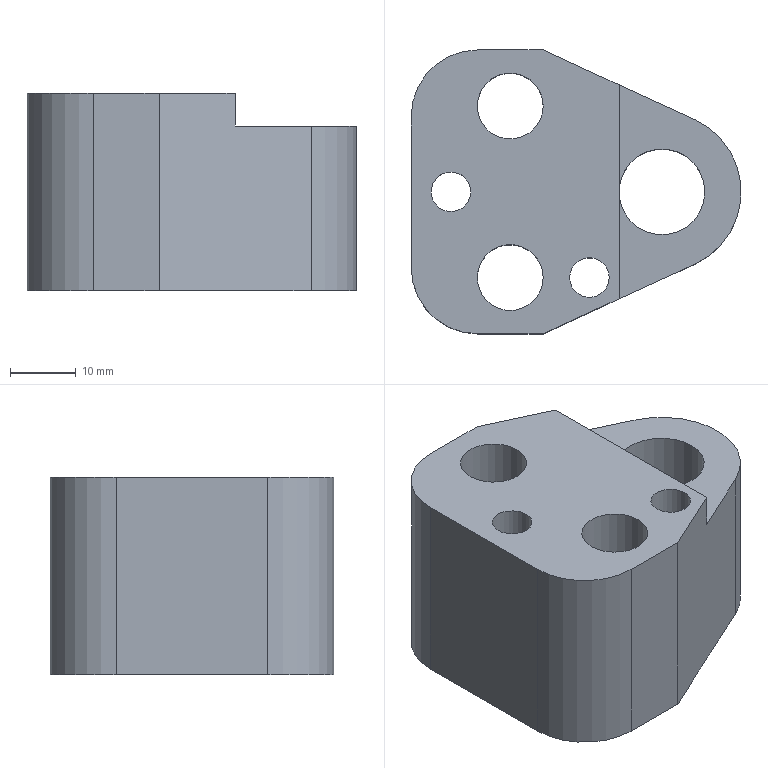Part | NX | features solid 2 | 1 solid | 25 faces | box 50 x 43 x 30 mm | volume 35945 mm3 | plane 13 | cylinder 12 | commonest cylinder face diameters 6 x2 8 x2 10 x2 14 x2 20 x2 13 x1
STEP:
#1=CARTESIAN_POINT('',(-1290.413,384.928,103.));
#2=VERTEX_POINT('',#1);
#3=CARTESIAN_POINT('',(-1294.413,384.928,103.));
#4=DIRECTION('',(0.,0.,1.));
#5=DIRECTION('',(1.,0.,0.));
#6=AXIS2_PLACEMENT_3D('',#3,#4,#5);
#7=CIRCLE('',#6,4.);
#8=EDGE_CURVE('',#2,#2,#7,.F.);
#9=ORIENTED_EDGE('',*,*,#8,.F.);
#10=EDGE_LOOP('',(#9));
#11=FACE_BOUND('',#10,.T.);
#12=CARTESIAN_POINT('',(-1292.413,371.928,103.));
#13=VERTEX_POINT('',#12);
#14=CARTESIAN_POINT('',(-1285.413,371.928,103.));
#15=DIRECTION('',(0.,0.,-1.));
#16=DIRECTION('',(-1.,0.,0.));
#17=AXIS2_PLACEMENT_3D('',#14,#15,#16);
#18=CIRCLE('',#17,7.);
#19=EDGE_CURVE('',#13,#13,#18,.T.);
#20=ORIENTED_EDGE('',*,*,#19,.F.);
#21=EDGE_LOOP('',(#20));
#22=FACE_BOUND('',#21,.T.);
#23=CARTESIAN_POINT('',(-1292.413,397.928,103.));
#24=VERTEX_POINT('',#23);
#25=CARTESIAN_POINT('',(-1285.413,397.928,103.));
#26=DIRECTION('',(0.,0.,-1.));
#27=DIRECTION('',(-1.,0.,0.));
#28=AXIS2_PLACEMENT_3D('',#25,#26,#27);
#29=CIRCLE('',#28,7.);
#30=EDGE_CURVE('',#24,#24,#29,.T.);
#31=ORIENTED_EDGE('',*,*,#30,.F.);
#32=EDGE_LOOP('',(#31));
#33=FACE_BOUND('',#32,.T.);
#34=CARTESIAN_POINT('',(-1255.913,384.928,103.));
#35=VERTEX_POINT('',#34);
#36=CARTESIAN_POINT('',(-1262.413,384.928,103.));
#37=DIRECTION('',(0.,0.,1.));
#38=DIRECTION('',(1.,0.,0.));
#39=AXIS2_PLACEMENT_3D('',#36,#37,#38);
#40=CIRCLE('',#39,6.5);
#41=EDGE_CURVE('',#35,#35,#40,.T.);
#42=ORIENTED_EDGE('',*,*,#41,.T.);
#43=EDGE_LOOP('',(#42));
#44=FACE_BOUND('',#43,.T.);
#45=CARTESIAN_POINT('',(-1257.394,395.828,103.));
#46=VERTEX_POINT('',#45);
#47=CARTESIAN_POINT('',(-1280.413,406.428,103.));
#48=VERTEX_POINT('',#47);
#49=CARTESIAN_POINT('',(-1257.394,395.828,103.));
#50=DIRECTION('',(-0.9083,0.4183,0.));
#51=VECTOR('',#50,1000.);
#52=LINE('',#49,#51);
#53=EDGE_CURVE('',#46,#48,#52,.T.);
#54=ORIENTED_EDGE('',*,*,#53,.F.);
#55=CARTESIAN_POINT('',(-1257.394,374.028,103.));
#56=VERTEX_POINT('',#55);
#57=CARTESIAN_POINT('',(-1262.413,384.928,103.));
#58=DIRECTION('',(0.,0.,-1.));
#59=DIRECTION('',(-1.,0.,0.));
#60=AXIS2_PLACEMENT_3D('',#57,#58,#59);
#61=CIRCLE('',#60,12.);
#62=EDGE_CURVE('',#46,#56,#61,.T.);
#63=ORIENTED_EDGE('',*,*,#62,.T.);
#64=CARTESIAN_POINT('',(-1280.413,363.428,103.));
#65=VERTEX_POINT('',#64);
#66=CARTESIAN_POINT('',(-1257.394,374.028,103.));
#67=DIRECTION('',(-0.9083,-0.4183,0.));
#68=VECTOR('',#67,1000.);
#69=LINE('',#66,#68);
#70=EDGE_CURVE('',#56,#65,#69,.T.);
#71=ORIENTED_EDGE('',*,*,#70,.T.);
#72=CARTESIAN_POINT('',(-1290.413,363.428,103.));
#73=VERTEX_POINT('',#72);
#74=CARTESIAN_POINT('',(-1280.413,363.428,103.));
#75=DIRECTION('',(-1.,0.,0.));
#76=VECTOR('',#75,1000.);
#77=LINE('',#74,#76);
#78=EDGE_CURVE('',#65,#73,#77,.T.);
#79=ORIENTED_EDGE('',*,*,#78,.T.);
#80=CARTESIAN_POINT('',(-1300.413,373.428,103.));
#81=VERTEX_POINT('',#80);
#82=CARTESIAN_POINT('',(-1290.413,373.428,103.));
#83=DIRECTION('',(0.,0.,-1.));
#84=DIRECTION('',(-1.,0.,0.));
#85=AXIS2_PLACEMENT_3D('',#82,#83,#84);
#86=CIRCLE('',#85,10.);
#87=EDGE_CURVE('',#73,#81,#86,.T.);
#88=ORIENTED_EDGE('',*,*,#87,.T.);
#89=CARTESIAN_POINT('',(-1300.413,396.428,103.));
#90=VERTEX_POINT('',#89);
#91=CARTESIAN_POINT('',(-1300.413,396.428,103.));
#92=DIRECTION('',(0.,-1.,0.));
#93=VECTOR('',#92,1000.);
#94=LINE('',#91,#93);
#95=EDGE_CURVE('',#90,#81,#94,.T.);
#96=ORIENTED_EDGE('',*,*,#95,.F.);
#97=CARTESIAN_POINT('',(-1290.413,406.428,103.));
#98=VERTEX_POINT('',#97);
#99=CARTESIAN_POINT('',(-1290.413,396.428,103.));
#100=DIRECTION('',(0.,0.,-1.));
#101=DIRECTION('',(-1.,0.,0.));
#102=AXIS2_PLACEMENT_3D('',#99,#100,#101);
#103=CIRCLE('',#102,10.);
#104=EDGE_CURVE('',#90,#98,#103,.T.);
#105=ORIENTED_EDGE('',*,*,#104,.T.);
#106=CARTESIAN_POINT('',(-1280.413,406.428,103.));
#107=DIRECTION('',(-1.,0.,0.));
#108=VECTOR('',#107,1000.);
#109=LINE('',#106,#108);
#110=EDGE_CURVE('',#48,#98,#109,.T.);
#111=ORIENTED_EDGE('',*,*,#110,.F.);
#112=EDGE_LOOP('',(#54,#63,#71,#79,#88,#96,#105,#111));
#113=FACE_BOUND('',#112,.T.);
#114=CARTESIAN_POINT('',(-1269.413,371.928,103.));
#115=VERTEX_POINT('',#114);
#116=CARTESIAN_POINT('',(-1273.413,371.928,103.));
#117=DIRECTION('',(0.,0.,1.));
#118=DIRECTION('',(1.,0.,0.));
#119=AXIS2_PLACEMENT_3D('',#116,#117,#118);
#120=CIRCLE('',#119,4.);
#121=EDGE_CURVE('',#115,#115,#120,.F.);
#122=ORIENTED_EDGE('',*,*,#121,.F.);
#123=EDGE_LOOP('',(#122));
#124=FACE_BOUND('',#123,.T.);
#125=CARTESIAN_POINT('',(-1290.413,396.428,103.));
#126=DIRECTION('',(0.,0.,-1.));
#127=DIRECTION('',(-1.,0.,0.));
#128=AXIS2_PLACEMENT_3D('',#125,#126,#127);
#129=PLANE('',#128);
#130=ADVANCED_FACE('',(#11,#22,#33,#44,#113,#124),#129,.T.);
#131=CARTESIAN_POINT('',(-1297.413,384.928,133.));
#132=VERTEX_POINT('',#131);
#133=CARTESIAN_POINT('',(-1294.413,384.928,133.));
#134=DIRECTION('',(0.,0.,-1.));
#135=DIRECTION('',(-1.,0.,0.));
#136=AXIS2_PLACEMENT_3D('',#133,#134,#135);
#137=CIRCLE('',#136,3.);
#138=EDGE_CURVE('',#132,#132,#137,.T.);
#139=ORIENTED_EDGE('',*,*,#138,.F.);
#140=EDGE_LOOP('',(#139));
#141=FACE_BOUND('',#140,.T.);
#142=CARTESIAN_POINT('',(-1297.413,384.928,123.));
#143=VERTEX_POINT('',#142);
#144=CARTESIAN_POINT('',(-1294.413,384.928,123.));
#145=DIRECTION('',(0.,0.,-1.));
#146=DIRECTION('',(-1.,0.,0.));
#147=AXIS2_PLACEMENT_3D('',#144,#145,#146);
#148=CIRCLE('',#147,3.);
#149=EDGE_CURVE('',#143,#143,#148,.T.);
#150=ORIENTED_EDGE('',*,*,#149,.T.);
#151=EDGE_LOOP('',(#150));
#152=FACE_BOUND('',#151,.T.);
#153=CARTESIAN_POINT('',(-1294.413,384.928,103.));
#154=DIRECTION('',(0.,0.,1.));
#155=DIRECTION('',(1.,0.,0.));
#156=AXIS2_PLACEMENT_3D('',#153,#154,#155);
#157=CYLINDRICAL_SURFACE('',#156,3.);
#158=ADVANCED_FACE('',(#141,#152),#157,.F.);
#159=CARTESIAN_POINT('',(-1290.413,371.928,133.));
#160=VERTEX_POINT('',#159);
#161=CARTESIAN_POINT('',(-1285.413,371.928,133.));
#162=DIRECTION('',(0.,0.,-1.));
#163=DIRECTION('',(-1.,0.,0.));
#164=AXIS2_PLACEMENT_3D('',#161,#162,#163);
#165=CIRCLE('',#164,5.);
#166=EDGE_CURVE('',#160,#160,#165,.T.);
#167=ORIENTED_EDGE('',*,*,#166,.F.);
#168=EDGE_LOOP('',(#167));
#169=FACE_BOUND('',#168,.T.);
#170=CARTESIAN_POINT('',(-1290.413,371.928,113.));
#171=VERTEX_POINT('',#170);
#172=CARTESIAN_POINT('',(-1285.413,371.928,113.));
#173=DIRECTION('',(0.,0.,-1.));
#174=DIRECTION('',(-1.,0.,0.));
#175=AXIS2_PLACEMENT_3D('',#172,#173,#174);
#176=CIRCLE('',#175,5.);
#177=EDGE_CURVE('',#171,#171,#176,.T.);
#178=ORIENTED_EDGE('',*,*,#177,.T.);
#179=EDGE_LOOP('',(#178));
#180=FACE_BOUND('',#179,.T.);
#181=CARTESIAN_POINT('',(-1285.413,371.928,103.));
#182=DIRECTION('',(0.,0.,1.));
#183=DIRECTION('',(1.,0.,0.));
#184=AXIS2_PLACEMENT_3D('',#181,#182,#183);
#185=CYLINDRICAL_SURFACE('',#184,5.);
#186=ADVANCED_FACE('',(#169,#180),#185,.F.);
#187=CARTESIAN_POINT('',(-1290.413,397.928,133.));
#188=VERTEX_POINT('',#187);
#189=CARTESIAN_POINT('',(-1285.413,397.928,133.));
#190=DIRECTION('',(0.,0.,-1.));
#191=DIRECTION('',(-1.,0.,0.));
#192=AXIS2_PLACEMENT_3D('',#189,#190,#191);
#193=CIRCLE('',#192,5.);
#194=EDGE_CURVE('',#188,#188,#193,.T.);
#195=ORIENTED_EDGE('',*,*,#194,.F.);
#196=EDGE_LOOP('',(#195));
#197=FACE_BOUND('',#196,.T.);
#198=CARTESIAN_POINT('',(-1290.413,397.928,113.));
#199=VERTEX_POINT('',#198);
#200=CARTESIAN_POINT('',(-1285.413,397.928,113.));
#201=DIRECTION('',(0.,0.,-1.));
#202=DIRECTION('',(-1.,0.,0.));
#203=AXIS2_PLACEMENT_3D('',#200,#201,#202);
#204=CIRCLE('',#203,5.);
#205=EDGE_CURVE('',#199,#199,#204,.T.);
#206=ORIENTED_EDGE('',*,*,#205,.T.);
#207=EDGE_LOOP('',(#206));
#208=FACE_BOUND('',#207,.T.);
#209=CARTESIAN_POINT('',(-1285.413,397.928,103.));
#210=DIRECTION('',(0.,0.,1.));
#211=DIRECTION('',(1.,0.,0.));
#212=AXIS2_PLACEMENT_3D('',#209,#210,#211);
#213=CYLINDRICAL_SURFACE('',#212,5.);
#214=ADVANCED_FACE('',(#197,#208),#213,.F.);
#215=CARTESIAN_POINT('',(-1276.413,371.928,133.));
#216=VERTEX_POINT('',#215);
#217=CARTESIAN_POINT('',(-1273.413,371.928,133.));
#218=DIRECTION('',(0.,0.,-1.));
#219=DIRECTION('',(-1.,0.,0.));
#220=AXIS2_PLACEMENT_3D('',#217,#218,#219);
#221=CIRCLE('',#220,3.);
#222=EDGE_CURVE('',#216,#216,#221,.T.);
#223=ORIENTED_EDGE('',*,*,#222,.T.);
#224=EDGE_LOOP('',(#223));
#225=FACE_BOUND('',#224,.T.);
#226=ORIENTED_EDGE('',*,*,#166,.T.);
#227=EDGE_LOOP('',(#226));
#228=FACE_BOUND('',#227,.T.);
#229=CARTESIAN_POINT('',(-1268.913,368.724,133.));
#230=VERTEX_POINT('',#229);
#231=CARTESIAN_POINT('',(-1280.413,363.428,133.));
#232=VERTEX_POINT('',#231);
#233=CARTESIAN_POINT('',(-1257.394,374.028,133.));
#234=DIRECTION('',(-0.9083,-0.4183,0.));
#235=VECTOR('',#234,1000.);
#236=LINE('',#233,#235);
#237=EDGE_CURVE('',#230,#232,#236,.T.);
#238=ORIENTED_EDGE('',*,*,#237,.F.);
#239=CARTESIAN_POINT('',(-1268.913,401.132,133.));
#240=VERTEX_POINT('',#239);
#241=CARTESIAN_POINT('',(-1268.913,401.132,133.));
#242=DIRECTION('',(0.,-1.,0.));
#243=VECTOR('',#242,1000.);
#244=LINE('',#241,#243);
#245=EDGE_CURVE('',#240,#230,#244,.T.);
#246=ORIENTED_EDGE('',*,*,#245,.F.);
#247=CARTESIAN_POINT('',(-1280.413,406.428,133.));
#248=VERTEX_POINT('',#247);
#249=CARTESIAN_POINT('',(-1257.394,395.828,133.));
#250=DIRECTION('',(-0.9083,0.4183,0.));
#251=VECTOR('',#250,1000.);
#252=LINE('',#249,#251);
#253=EDGE_CURVE('',#240,#248,#252,.T.);
#254=ORIENTED_EDGE('',*,*,#253,.T.);
#255=CARTESIAN_POINT('',(-1290.413,406.428,133.));
#256=VERTEX_POINT('',#255);
#257=CARTESIAN_POINT('',(-1280.413,406.428,133.));
#258=DIRECTION('',(-1.,0.,0.));
#259=VECTOR('',#258,1000.);
#260=LINE('',#257,#259);
#261=EDGE_CURVE('',#248,#256,#260,.T.);
#262=ORIENTED_EDGE('',*,*,#261,.T.);
#263=CARTESIAN_POINT('',(-1300.413,396.428,133.));
#264=VERTEX_POINT('',#263);
#265=CARTESIAN_POINT('',(-1290.413,396.428,133.));
#266=DIRECTION('',(0.,0.,-1.));
#267=DIRECTION('',(-1.,0.,0.));
#268=AXIS2_PLACEMENT_3D('',#265,#266,#267);
#269=CIRCLE('',#268,10.);
#270=EDGE_CURVE('',#264,#256,#269,.T.);
#271=ORIENTED_EDGE('',*,*,#270,.F.);
#272=CARTESIAN_POINT('',(-1300.413,373.428,133.));
#273=VERTEX_POINT('',#272);
#274=CARTESIAN_POINT('',(-1300.413,396.428,133.));
#275=DIRECTION('',(0.,-1.,0.));
#276=VECTOR('',#275,1000.);
#277=LINE('',#274,#276);
#278=EDGE_CURVE('',#264,#273,#277,.T.);
#279=ORIENTED_EDGE('',*,*,#278,.T.);
#280=CARTESIAN_POINT('',(-1290.413,363.428,133.));
#281=VERTEX_POINT('',#280);
#282=CARTESIAN_POINT('',(-1290.413,373.428,133.));
#283=DIRECTION('',(0.,0.,-1.));
#284=DIRECTION('',(-1.,0.,0.));
#285=AXIS2_PLACEMENT_3D('',#282,#283,#284);
#286=CIRCLE('',#285,10.);
#287=EDGE_CURVE('',#281,#273,#286,.T.);
#288=ORIENTED_EDGE('',*,*,#287,.F.);
#289=CARTESIAN_POINT('',(-1280.413,363.428,133.));
#290=DIRECTION('',(-1.,0.,0.));
#291=VECTOR('',#290,1000.);
#292=LINE('',#289,#291);
#293=EDGE_CURVE('',#232,#281,#292,.T.);
#294=ORIENTED_EDGE('',*,*,#293,.F.);
#295=EDGE_LOOP('',(#238,#246,#254,#262,#271,#279,#288,#294));
#296=FACE_BOUND('',#295,.T.);
#297=ORIENTED_EDGE('',*,*,#194,.T.);
#298=EDGE_LOOP('',(#297));
#299=FACE_BOUND('',#298,.T.);
#300=ORIENTED_EDGE('',*,*,#138,.T.);
#301=EDGE_LOOP('',(#300));
#302=FACE_BOUND('',#301,.T.);
#303=CARTESIAN_POINT('',(-1290.413,396.428,133.));
#304=DIRECTION('',(0.,0.,-1.));
#305=DIRECTION('',(-1.,0.,0.));
#306=AXIS2_PLACEMENT_3D('',#303,#304,#305);
#307=PLANE('',#306);
#308=ADVANCED_FACE('',(#225,#228,#296,#299,#302),#307,.F.);
#309=CARTESIAN_POINT('',(-1268.913,401.132,128.));
#310=VERTEX_POINT('',#309);
#311=CARTESIAN_POINT('',(-1268.913,401.132,128.));
#312=DIRECTION('',(0.,0.,1.));
#313=VECTOR('',#312,1000.);
#314=LINE('',#311,#313);
#315=EDGE_CURVE('',#310,#240,#314,.T.);
#316=ORIENTED_EDGE('',*,*,#315,.F.);
#317=CARTESIAN_POINT('',(-1257.394,395.828,128.));
#318=VERTEX_POINT('',#317);
#319=CARTESIAN_POINT('',(-1268.913,401.132,128.));
#320=DIRECTION('',(0.9083,-0.4183,0.));
#321=VECTOR('',#320,1000.);
#322=LINE('',#319,#321);
#323=EDGE_CURVE('',#310,#318,#322,.T.);
#324=ORIENTED_EDGE('',*,*,#323,.T.);
#325=CARTESIAN_POINT('',(-1257.394,395.828,103.));
#326=DIRECTION('',(0.,0.,1.));
#327=VECTOR('',#326,1000.);
#328=LINE('',#325,#327);
#329=EDGE_CURVE('',#46,#318,#328,.T.);
#330=ORIENTED_EDGE('',*,*,#329,.F.);
#331=ORIENTED_EDGE('',*,*,#53,.T.);
#332=CARTESIAN_POINT('',(-1280.413,406.428,103.));
#333=DIRECTION('',(0.,0.,1.));
#334=VECTOR('',#333,1000.);
#335=LINE('',#332,#334);
#336=EDGE_CURVE('',#48,#248,#335,.T.);
#337=ORIENTED_EDGE('',*,*,#336,.T.);
#338=ORIENTED_EDGE('',*,*,#253,.F.);
#339=EDGE_LOOP('',(#316,#324,#330,#331,#337,#338));
#340=FACE_BOUND('',#339,.T.);
#341=CARTESIAN_POINT('',(-1257.394,395.828,103.));
#342=DIRECTION('',(0.4183,0.9083,0.));
#343=DIRECTION('',(-0.9083,0.4183,0.));
#344=AXIS2_PLACEMENT_3D('',#341,#342,#343);
#345=PLANE('',#344);
#346=ADVANCED_FACE('',(#340),#345,.T.);
#347=ORIENTED_EDGE('',*,*,#261,.F.);
#348=ORIENTED_EDGE('',*,*,#336,.F.);
#349=ORIENTED_EDGE('',*,*,#110,.T.);
#350=CARTESIAN_POINT('',(-1290.413,406.428,103.));
#351=DIRECTION('',(0.,0.,1.));
#352=VECTOR('',#351,1000.);
#353=LINE('',#350,#352);
#354=EDGE_CURVE('',#98,#256,#353,.T.);
#355=ORIENTED_EDGE('',*,*,#354,.T.);
#356=EDGE_LOOP('',(#347,#348,#349,#355));
#357=FACE_BOUND('',#356,.T.);
#358=CARTESIAN_POINT('',(-1280.413,406.428,103.));
#359=DIRECTION('',(0.,1.,0.));
#360=DIRECTION('',(-1.,0.,0.));
#361=AXIS2_PLACEMENT_3D('',#358,#359,#360);
#362=PLANE('',#361);
#363=ADVANCED_FACE('',(#357),#362,.T.);
#364=ORIENTED_EDGE('',*,*,#270,.T.);
#365=ORIENTED_EDGE('',*,*,#354,.F.);
#366=ORIENTED_EDGE('',*,*,#104,.F.);
#367=CARTESIAN_POINT('',(-1300.413,396.428,103.));
#368=DIRECTION('',(0.,0.,1.));
#369=VECTOR('',#368,1000.);
#370=LINE('',#367,#369);
#371=EDGE_CURVE('',#90,#264,#370,.T.);
#372=ORIENTED_EDGE('',*,*,#371,.T.);
#373=EDGE_LOOP('',(#364,#365,#366,#372));
#374=FACE_BOUND('',#373,.T.);
#375=CARTESIAN_POINT('',(-1290.413,396.428,103.));
#376=DIRECTION('',(0.,0.,1.));
#377=DIRECTION('',(1.,0.,0.));
#378=AXIS2_PLACEMENT_3D('',#375,#376,#377);
#379=CYLINDRICAL_SURFACE('',#378,10.);
#380=ADVANCED_FACE('',(#374),#379,.T.);
#381=ORIENTED_EDGE('',*,*,#278,.F.);
#382=ORIENTED_EDGE('',*,*,#371,.F.);
#383=ORIENTED_EDGE('',*,*,#95,.T.);
#384=CARTESIAN_POINT('',(-1300.413,373.428,103.));
#385=DIRECTION('',(0.,0.,1.));
#386=VECTOR('',#385,1000.);
#387=LINE('',#384,#386);
#388=EDGE_CURVE('',#81,#273,#387,.T.);
#389=ORIENTED_EDGE('',*,*,#388,.T.);
#390=EDGE_LOOP('',(#381,#382,#383,#389));
#391=FACE_BOUND('',#390,.T.);
#392=CARTESIAN_POINT('',(-1300.413,396.428,103.));
#393=DIRECTION('',(-1.,0.,0.));
#394=DIRECTION('',(0.,-1.,0.));
#395=AXIS2_PLACEMENT_3D('',#392,#393,#394);
#396=PLANE('',#395);
#397=ADVANCED_FACE('',(#391),#396,.T.);
#398=ORIENTED_EDGE('',*,*,#287,.T.);
#399=ORIENTED_EDGE('',*,*,#388,.F.);
#400=ORIENTED_EDGE('',*,*,#87,.F.);
#401=CARTESIAN_POINT('',(-1290.413,363.428,103.));
#402=DIRECTION('',(0.,0.,1.));
#403=VECTOR('',#402,1000.);
#404=LINE('',#401,#403);
#405=EDGE_CURVE('',#73,#281,#404,.T.);
#406=ORIENTED_EDGE('',*,*,#405,.T.);
#407=EDGE_LOOP('',(#398,#399,#400,#406));
#408=FACE_BOUND('',#407,.T.);
#409=CARTESIAN_POINT('',(-1290.413,373.428,103.));
#410=DIRECTION('',(0.,0.,1.));
#411=DIRECTION('',(1.,0.,0.));
#412=AXIS2_PLACEMENT_3D('',#409,#410,#411);
#413=CYLINDRICAL_SURFACE('',#412,10.);
#414=ADVANCED_FACE('',(#408),#413,.T.);
#415=ORIENTED_EDGE('',*,*,#293,.T.);
#416=ORIENTED_EDGE('',*,*,#405,.F.);
#417=ORIENTED_EDGE('',*,*,#78,.F.);
#418=CARTESIAN_POINT('',(-1280.413,363.428,103.));
#419=DIRECTION('',(0.,0.,1.));
#420=VECTOR('',#419,1000.);
#421=LINE('',#418,#420);
#422=EDGE_CURVE('',#65,#232,#421,.T.);
#423=ORIENTED_EDGE('',*,*,#422,.T.);
#424=EDGE_LOOP('',(#415,#416,#417,#423));
#425=FACE_BOUND('',#424,.T.);
#426=CARTESIAN_POINT('',(-1280.413,363.428,103.));
#427=DIRECTION('',(0.,1.,0.));
#428=DIRECTION('',(-1.,0.,0.));
#429=AXIS2_PLACEMENT_3D('',#426,#427,#428);
#430=PLANE('',#429);
#431=ADVANCED_FACE('',(#425),#430,.F.);
#432=CARTESIAN_POINT('',(-1268.913,368.724,128.));
#433=VERTEX_POINT('',#432);
#434=CARTESIAN_POINT('',(-1257.394,374.028,128.));
#435=VERTEX_POINT('',#434);
#436=CARTESIAN_POINT('',(-1268.913,368.724,128.));
#437=DIRECTION('',(0.9083,0.4183,0.));
#438=VECTOR('',#437,1000.);
#439=LINE('',#436,#438);
#440=EDGE_CURVE('',#433,#435,#439,.T.);
#441=ORIENTED_EDGE('',*,*,#440,.F.);
#442=CARTESIAN_POINT('',(-1268.913,368.724,128.));
#443=DIRECTION('',(0.,0.,1.));
#444=VECTOR('',#443,1000.);
#445=LINE('',#442,#444);
#446=EDGE_CURVE('',#433,#230,#445,.T.);
#447=ORIENTED_EDGE('',*,*,#446,.T.);
#448=ORIENTED_EDGE('',*,*,#237,.T.);
#449=ORIENTED_EDGE('',*,*,#422,.F.);
#450=ORIENTED_EDGE('',*,*,#70,.F.);
#451=CARTESIAN_POINT('',(-1257.394,374.028,103.));
#452=DIRECTION('',(0.,0.,1.));
#453=VECTOR('',#452,1000.);
#454=LINE('',#451,#453);
#455=EDGE_CURVE('',#56,#435,#454,.T.);
#456=ORIENTED_EDGE('',*,*,#455,.T.);
#457=EDGE_LOOP('',(#441,#447,#448,#449,#450,#456));
#458=FACE_BOUND('',#457,.T.);
#459=CARTESIAN_POINT('',(-1257.394,374.028,103.));
#460=DIRECTION('',(-0.4183,0.9083,0.));
#461=DIRECTION('',(-0.9083,-0.4183,0.));
#462=AXIS2_PLACEMENT_3D('',#459,#460,#461);
#463=PLANE('',#462);
#464=ADVANCED_FACE('',(#458),#463,.F.);
#465=ORIENTED_EDGE('',*,*,#329,.T.);
#466=CARTESIAN_POINT('',(-1262.413,384.928,128.));
#467=DIRECTION('',(0.,0.,-1.));
#468=DIRECTION('',(-1.,0.,0.));
#469=AXIS2_PLACEMENT_3D('',#466,#467,#468);
#470=CIRCLE('',#469,12.);
#471=EDGE_CURVE('',#318,#435,#470,.T.);
#472=ORIENTED_EDGE('',*,*,#471,.T.);
#473=ORIENTED_EDGE('',*,*,#455,.F.);
#474=ORIENTED_EDGE('',*,*,#62,.F.);
#475=EDGE_LOOP('',(#465,#472,#473,#474));
#476=FACE_BOUND('',#475,.T.);
#477=CARTESIAN_POINT('',(-1262.413,384.928,103.));
#478=DIRECTION('',(0.,0.,1.));
#479=DIRECTION('',(1.,0.,0.));
#480=AXIS2_PLACEMENT_3D('',#477,#478,#479);
#481=CYLINDRICAL_SURFACE('',#480,12.);
#482=ADVANCED_FACE('',(#476),#481,.T.);
#483=CARTESIAN_POINT('',(-1268.913,384.928,128.));
#484=VERTEX_POINT('',#483);
#485=CARTESIAN_POINT('',(-1262.413,384.928,128.));
#486=DIRECTION('',(0.,0.,-1.));
#487=DIRECTION('',(-1.,0.,0.));
#488=AXIS2_PLACEMENT_3D('',#485,#486,#487);
#489=CIRCLE('',#488,6.5);
#490=EDGE_CURVE('',#484,#484,#489,.F.);
#491=ORIENTED_EDGE('',*,*,#490,.T.);
#492=EDGE_LOOP('',(#491));
#493=FACE_BOUND('',#492,.T.);
#494=ORIENTED_EDGE('',*,*,#41,.F.);
#495=EDGE_LOOP('',(#494));
#496=FACE_BOUND('',#495,.T.);
#497=CARTESIAN_POINT('',(-1262.413,384.928,103.));
#498=DIRECTION('',(0.,0.,1.));
#499=DIRECTION('',(1.,0.,0.));
#500=AXIS2_PLACEMENT_3D('',#497,#498,#499);
#501=CYLINDRICAL_SURFACE('',#500,6.5);
#502=ADVANCED_FACE('',(#493,#496),#501,.F.);
#503=ORIENTED_EDGE('',*,*,#245,.T.);
#504=ORIENTED_EDGE('',*,*,#446,.F.);
#505=CARTESIAN_POINT('',(-1268.913,401.132,128.));
#506=DIRECTION('',(0.,-1.,0.));
#507=VECTOR('',#506,1000.);
#508=LINE('',#505,#507);
#509=EDGE_CURVE('',#484,#433,#508,.T.);
#510=ORIENTED_EDGE('',*,*,#509,.F.);
#511=CARTESIAN_POINT('',(-1268.913,401.132,128.));
#512=DIRECTION('',(0.,-1.,0.));
#513=VECTOR('',#512,1000.);
#514=LINE('',#511,#513);
#515=EDGE_CURVE('',#310,#484,#514,.T.);
#516=ORIENTED_EDGE('',*,*,#515,.F.);
#517=ORIENTED_EDGE('',*,*,#315,.T.);
#518=EDGE_LOOP('',(#503,#504,#510,#516,#517));
#519=FACE_BOUND('',#518,.T.);
#520=CARTESIAN_POINT('',(-1268.913,401.132,128.));
#521=DIRECTION('',(-1.,0.,0.));
#522=DIRECTION('',(0.,-1.,0.));
#523=AXIS2_PLACEMENT_3D('',#520,#521,#522);
#524=PLANE('',#523);
#525=ADVANCED_FACE('',(#519),#524,.F.);
#526=ORIENTED_EDGE('',*,*,#509,.T.);
#527=ORIENTED_EDGE('',*,*,#440,.T.);
#528=ORIENTED_EDGE('',*,*,#471,.F.);
#529=ORIENTED_EDGE('',*,*,#323,.F.);
#530=ORIENTED_EDGE('',*,*,#515,.T.);
#531=ORIENTED_EDGE('',*,*,#490,.F.);
#532=EDGE_LOOP('',(#526,#527,#528,#529,#530,#531));
#533=FACE_BOUND('',#532,.T.);
#534=CARTESIAN_POINT('',(-1262.413,384.928,128.));
#535=DIRECTION('',(0.,0.,-1.));
#536=DIRECTION('',(-1.,0.,0.));
#537=AXIS2_PLACEMENT_3D('',#534,#535,#536);
#538=PLANE('',#537);
#539=ADVANCED_FACE('',(#533),#538,.F.);
#540=CARTESIAN_POINT('',(-1276.413,371.928,123.));
#541=VERTEX_POINT('',#540);
#542=CARTESIAN_POINT('',(-1273.413,371.928,123.));
#543=DIRECTION('',(0.,0.,-1.));
#544=DIRECTION('',(-1.,0.,0.));
#545=AXIS2_PLACEMENT_3D('',#542,#543,#544);
#546=CIRCLE('',#545,3.);
#547=EDGE_CURVE('',#541,#541,#546,.T.);
#548=ORIENTED_EDGE('',*,*,#547,.T.);
#549=EDGE_LOOP('',(#548));
#550=FACE_BOUND('',#549,.T.);
#551=ORIENTED_EDGE('',*,*,#222,.F.);
#552=EDGE_LOOP('',(#551));
#553=FACE_BOUND('',#552,.T.);
#554=CARTESIAN_POINT('',(-1273.413,371.928,103.));
#555=DIRECTION('',(0.,0.,1.));
#556=DIRECTION('',(1.,0.,0.));
#557=AXIS2_PLACEMENT_3D('',#554,#555,#556);
#558=CYLINDRICAL_SURFACE('',#557,3.);
#559=ADVANCED_FACE('',(#550,#553),#558,.F.);
#560=CARTESIAN_POINT('',(-1292.413,397.928,113.));
#561=VERTEX_POINT('',#560);
#562=CARTESIAN_POINT('',(-1285.413,397.928,113.));
#563=DIRECTION('',(0.,0.,-1.));
#564=DIRECTION('',(-1.,0.,0.));
#565=AXIS2_PLACEMENT_3D('',#562,#563,#564);
#566=CIRCLE('',#565,7.);
#567=EDGE_CURVE('',#561,#561,#566,.T.);
#568=ORIENTED_EDGE('',*,*,#567,.F.);
#569=EDGE_LOOP('',(#568));
#570=FACE_BOUND('',#569,.T.);
#571=ORIENTED_EDGE('',*,*,#30,.T.);
#572=EDGE_LOOP('',(#571));
#573=FACE_BOUND('',#572,.T.);
#574=CARTESIAN_POINT('',(-1285.413,397.928,113.));
#575=DIRECTION('',(0.,0.,-1.));
#576=DIRECTION('',(-1.,0.,0.));
#577=AXIS2_PLACEMENT_3D('',#574,#575,#576);
#578=CYLINDRICAL_SURFACE('',#577,7.);
#579=ADVANCED_FACE('',(#570,#573),#578,.F.);
#580=ORIENTED_EDGE('',*,*,#205,.F.);
#581=EDGE_LOOP('',(#580));
#582=FACE_BOUND('',#581,.T.);
#583=ORIENTED_EDGE('',*,*,#567,.T.);
#584=EDGE_LOOP('',(#583));
#585=FACE_BOUND('',#584,.T.);
#586=CARTESIAN_POINT('',(-1285.413,397.928,113.));
#587=DIRECTION('',(0.,0.,-1.));
#588=DIRECTION('',(-1.,0.,0.));
#589=AXIS2_PLACEMENT_3D('',#586,#587,#588);
#590=PLANE('',#589);
#591=ADVANCED_FACE('',(#582,#585),#590,.T.);
#592=CARTESIAN_POINT('',(-1292.413,371.928,113.));
#593=VERTEX_POINT('',#592);
#594=CARTESIAN_POINT('',(-1285.413,371.928,113.));
#595=DIRECTION('',(0.,0.,-1.));
#596=DIRECTION('',(-1.,0.,0.));
#597=AXIS2_PLACEMENT_3D('',#594,#595,#596);
#598=CIRCLE('',#597,7.);
#599=EDGE_CURVE('',#593,#593,#598,.T.);
#600=ORIENTED_EDGE('',*,*,#599,.F.);
#601=EDGE_LOOP('',(#600));
#602=FACE_BOUND('',#601,.T.);
#603=ORIENTED_EDGE('',*,*,#19,.T.);
#604=EDGE_LOOP('',(#603));
#605=FACE_BOUND('',#604,.T.);
#606=CARTESIAN_POINT('',(-1285.413,371.928,113.));
#607=DIRECTION('',(0.,0.,-1.));
#608=DIRECTION('',(-1.,0.,0.));
#609=AXIS2_PLACEMENT_3D('',#606,#607,#608);
#610=CYLINDRICAL_SURFACE('',#609,7.);
#611=ADVANCED_FACE('',(#602,#605),#610,.F.);
#612=ORIENTED_EDGE('',*,*,#177,.F.);
#613=EDGE_LOOP('',(#612));
#614=FACE_BOUND('',#613,.T.);
#615=ORIENTED_EDGE('',*,*,#599,.T.);
#616=EDGE_LOOP('',(#615));
#617=FACE_BOUND('',#616,.T.);
#618=CARTESIAN_POINT('',(-1285.413,371.928,113.));
#619=DIRECTION('',(0.,0.,-1.));
#620=DIRECTION('',(-1.,0.,0.));
#621=AXIS2_PLACEMENT_3D('',#618,#619,#620);
#622=PLANE('',#621);
#623=ADVANCED_FACE('',(#614,#617),#622,.T.);
#624=ORIENTED_EDGE('',*,*,#149,.F.);
#625=EDGE_LOOP('',(#624));
#626=FACE_BOUND('',#625,.T.);
#627=CARTESIAN_POINT('',(-1290.413,384.928,123.));
#628=VERTEX_POINT('',#627);
#629=CARTESIAN_POINT('',(-1294.413,384.928,123.));
#630=DIRECTION('',(0.,0.,1.));
#631=DIRECTION('',(1.,0.,0.));
#632=AXIS2_PLACEMENT_3D('',#629,#630,#631);
#633=CIRCLE('',#632,4.);
#634=EDGE_CURVE('',#628,#628,#633,.F.);
#635=ORIENTED_EDGE('',*,*,#634,.T.);
#636=EDGE_LOOP('',(#635));
#637=FACE_BOUND('',#636,.T.);
#638=CARTESIAN_POINT('',(-1294.413,384.928,123.));
#639=DIRECTION('',(0.,0.,1.));
#640=DIRECTION('',(1.,0.,0.));
#641=AXIS2_PLACEMENT_3D('',#638,#639,#640);
#642=PLANE('',#641);
#643=ADVANCED_FACE('',(#626,#637),#642,.F.);
#644=ORIENTED_EDGE('',*,*,#634,.F.);
#645=EDGE_LOOP('',(#644));
#646=FACE_BOUND('',#645,.T.);
#647=ORIENTED_EDGE('',*,*,#8,.T.);
#648=EDGE_LOOP('',(#647));
#649=FACE_BOUND('',#648,.T.);
#650=CARTESIAN_POINT('',(-1294.413,384.928,103.));
#651=DIRECTION('',(0.,0.,1.));
#652=DIRECTION('',(1.,0.,0.));
#653=AXIS2_PLACEMENT_3D('',#650,#651,#652);
#654=CYLINDRICAL_SURFACE('',#653,4.);
#655=ADVANCED_FACE('',(#646,#649),#654,.F.);
#656=ORIENTED_EDGE('',*,*,#547,.F.);
#657=EDGE_LOOP('',(#656));
#658=FACE_BOUND('',#657,.T.);
#659=CARTESIAN_POINT('',(-1269.413,371.928,123.));
#660=VERTEX_POINT('',#659);
#661=CARTESIAN_POINT('',(-1273.413,371.928,123.));
#662=DIRECTION('',(0.,0.,1.));
#663=DIRECTION('',(1.,0.,0.));
#664=AXIS2_PLACEMENT_3D('',#661,#662,#663);
#665=CIRCLE('',#664,4.);
#666=EDGE_CURVE('',#660,#660,#665,.F.);
#667=ORIENTED_EDGE('',*,*,#666,.T.);
#668=EDGE_LOOP('',(#667));
#669=FACE_BOUND('',#668,.T.);
#670=CARTESIAN_POINT('',(-1273.413,371.928,123.));
#671=DIRECTION('',(0.,0.,1.));
#672=DIRECTION('',(1.,0.,0.));
#673=AXIS2_PLACEMENT_3D('',#670,#671,#672);
#674=PLANE('',#673);
#675=ADVANCED_FACE('',(#658,#669),#674,.F.);
#676=ORIENTED_EDGE('',*,*,#666,.F.);
#677=EDGE_LOOP('',(#676));
#678=FACE_BOUND('',#677,.T.);
#679=ORIENTED_EDGE('',*,*,#121,.T.);
#680=EDGE_LOOP('',(#679));
#681=FACE_BOUND('',#680,.T.);
#682=CARTESIAN_POINT('',(-1273.413,371.928,103.));
#683=DIRECTION('',(0.,0.,1.));
#684=DIRECTION('',(1.,0.,0.));
#685=AXIS2_PLACEMENT_3D('',#682,#683,#684);
#686=CYLINDRICAL_SURFACE('',#685,4.);
#687=ADVANCED_FACE('',(#678,#681),#686,.F.);
#688=CLOSED_SHELL('',(#130,#158,#186,#214,#308,#346,#363,#380,#397,#414,#431,#464,#482,#502,#525,#539,#559,#579,#591,#611,#623,#643,#655,#675,#687));
#689=MANIFOLD_SOLID_BREP('',#688);
#690=(LENGTH_UNIT()NAMED_UNIT(*)SI_UNIT(.MILLI.,.METRE.));
#691=UNCERTAINTY_MEASURE_WITH_UNIT(LENGTH_MEASURE(0.00001),#690,'','');
#692=(NAMED_UNIT(*)PLANE_ANGLE_UNIT()SI_UNIT($,.RADIAN.));
#693=(NAMED_UNIT(*)SI_UNIT($,.STERADIAN.)SOLID_ANGLE_UNIT());
#694=(GEOMETRIC_REPRESENTATION_CONTEXT(3)GLOBAL_UNCERTAINTY_ASSIGNED_CONTEXT((#691))GLOBAL_UNIT_ASSIGNED_CONTEXT((#690,#692,#693))REPRESENTATION_CONTEXT('',''));
#695=ADVANCED_BREP_SHAPE_REPRESENTATION('',(#689),#694);